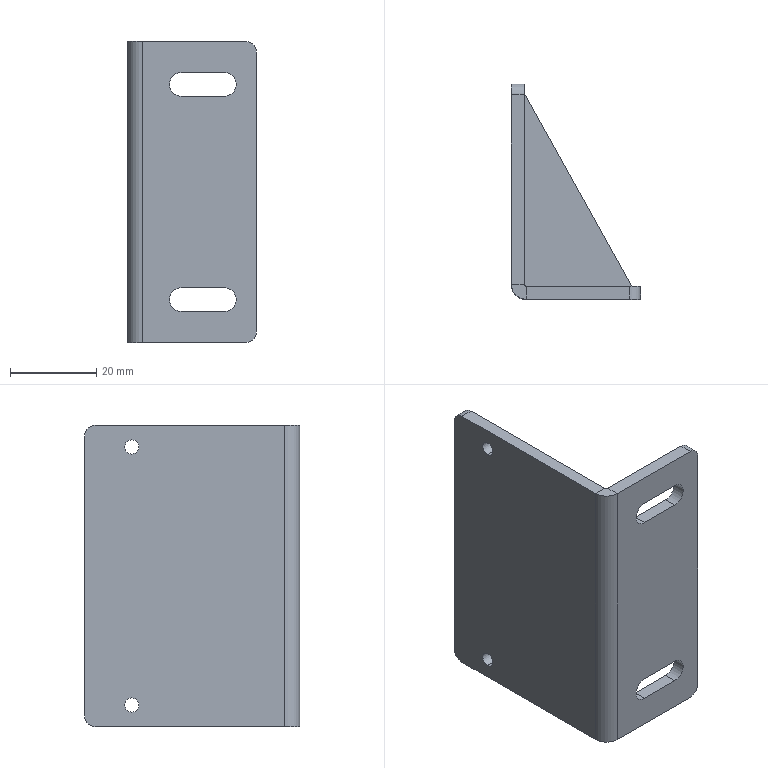Part | STEP file | KF-2212-070-007 | 2 solids | 35 faces | box 30 x 50 x 70 mm | volume 17137 mm3 | plane 21 | cylinder 14 | commonest cylinder face diameters 3.3 x4 5 x4 5.5 x4 1 x1 7 x1
STEP:
#1=CARTESIAN_POINT('',(3.,48.,36.5));
#2=VERTEX_POINT('',#1);
#3=CARTESIAN_POINT('',(28.,3.,36.5));
#4=VERTEX_POINT('',#3);
#5=CARTESIAN_POINT('',(3.,48.,36.5));
#6=DIRECTION('',(0.4856,-0.8742,0.));
#7=VECTOR('',#6,1000.);
#8=LINE('',#5,#7);
#9=EDGE_CURVE('',#2,#4,#8,.T.);
#10=ORIENTED_EDGE('',*,*,#9,.T.);
#11=CARTESIAN_POINT('',(28.,3.,33.5));
#12=VERTEX_POINT('',#11);
#13=CARTESIAN_POINT('',(28.,3.,33.5));
#14=DIRECTION('',(0.,0.,1.));
#15=VECTOR('',#14,1000.);
#16=LINE('',#13,#15);
#17=EDGE_CURVE('',#12,#4,#16,.T.);
#18=ORIENTED_EDGE('',*,*,#17,.F.);
#19=CARTESIAN_POINT('',(3.,48.,33.5));
#20=VERTEX_POINT('',#19);
#21=CARTESIAN_POINT('',(3.,48.,33.5));
#22=DIRECTION('',(0.4856,-0.8742,0.));
#23=VECTOR('',#22,1000.);
#24=LINE('',#21,#23);
#25=EDGE_CURVE('',#20,#12,#24,.T.);
#26=ORIENTED_EDGE('',*,*,#25,.F.);
#27=CARTESIAN_POINT('',(3.,48.,33.5));
#28=DIRECTION('',(0.,0.,1.));
#29=VECTOR('',#28,1000.);
#30=LINE('',#27,#29);
#31=EDGE_CURVE('',#20,#2,#30,.T.);
#32=ORIENTED_EDGE('',*,*,#31,.T.);
#33=EDGE_LOOP('',(#10,#18,#26,#32));
#34=FACE_OUTER_BOUND('',#33,.T.);
#35=CARTESIAN_POINT('',(3.,48.,33.5));
#36=DIRECTION('',(-0.8742,-0.4856,0.));
#37=DIRECTION('',(0.4856,-0.8742,0.));
#38=AXIS2_PLACEMENT_3D('',#35,#36,#37);
#39=PLANE('',#38);
#40=ADVANCED_FACE('',(#34),#39,.F.);
#41=CARTESIAN_POINT('',(3.,3.,36.5));
#42=VERTEX_POINT('',#41);
#43=CARTESIAN_POINT('',(3.,3.,36.5));
#44=DIRECTION('',(-1.,0.,0.));
#45=VECTOR('',#44,1000.);
#46=LINE('',#43,#45);
#47=EDGE_CURVE('',#4,#42,#46,.T.);
#48=ORIENTED_EDGE('',*,*,#47,.T.);
#49=CARTESIAN_POINT('',(3.,3.,33.5));
#50=VERTEX_POINT('',#49);
#51=CARTESIAN_POINT('',(3.,3.,33.5));
#52=DIRECTION('',(0.,0.,1.));
#53=VECTOR('',#52,1000.);
#54=LINE('',#51,#53);
#55=EDGE_CURVE('',#50,#42,#54,.T.);
#56=ORIENTED_EDGE('',*,*,#55,.F.);
#57=CARTESIAN_POINT('',(3.,3.,33.5));
#58=DIRECTION('',(-1.,0.,0.));
#59=VECTOR('',#58,1000.);
#60=LINE('',#57,#59);
#61=EDGE_CURVE('',#12,#50,#60,.T.);
#62=ORIENTED_EDGE('',*,*,#61,.F.);
#63=ORIENTED_EDGE('',*,*,#17,.T.);
#64=EDGE_LOOP('',(#48,#56,#62,#63));
#65=FACE_OUTER_BOUND('',#64,.T.);
#66=CARTESIAN_POINT('',(3.,3.,33.5));
#67=DIRECTION('',(0.,1.,0.));
#68=DIRECTION('',(0.,0.,1.));
#69=AXIS2_PLACEMENT_3D('',#66,#67,#68);
#70=PLANE('',#69);
#71=ADVANCED_FACE('',(#65),#70,.F.);
#72=CARTESIAN_POINT('',(3.,3.,36.5));
#73=DIRECTION('',(0.,1.,0.));
#74=VECTOR('',#73,1000.);
#75=LINE('',#72,#74);
#76=EDGE_CURVE('',#42,#2,#75,.T.);
#77=ORIENTED_EDGE('',*,*,#76,.T.);
#78=ORIENTED_EDGE('',*,*,#31,.F.);
#79=CARTESIAN_POINT('',(3.,3.,33.5));
#80=DIRECTION('',(0.,1.,0.));
#81=VECTOR('',#80,1000.);
#82=LINE('',#79,#81);
#83=EDGE_CURVE('',#50,#20,#82,.T.);
#84=ORIENTED_EDGE('',*,*,#83,.F.);
#85=ORIENTED_EDGE('',*,*,#55,.T.);
#86=EDGE_LOOP('',(#77,#78,#84,#85));
#87=FACE_OUTER_BOUND('',#86,.T.);
#88=CARTESIAN_POINT('',(3.,3.,33.5));
#89=DIRECTION('',(1.,0.,0.));
#90=DIRECTION('',(0.,0.,-1.));
#91=AXIS2_PLACEMENT_3D('',#88,#89,#90);
#92=PLANE('',#91);
#93=ADVANCED_FACE('',(#87),#92,.F.);
#94=ORIENTED_EDGE('',*,*,#25,.T.);
#95=ORIENTED_EDGE('',*,*,#61,.T.);
#96=ORIENTED_EDGE('',*,*,#83,.T.);
#97=EDGE_LOOP('',(#94,#95,#96));
#98=FACE_OUTER_BOUND('',#97,.T.);
#99=CARTESIAN_POINT('',(0.,0.,33.5));
#100=DIRECTION('',(0.,0.,1.));
#101=DIRECTION('',(1.,0.,0.));
#102=AXIS2_PLACEMENT_3D('',#99,#100,#101);
#103=PLANE('',#102);
#104=ADVANCED_FACE('',(#98),#103,.F.);
#105=ORIENTED_EDGE('',*,*,#9,.F.);
#106=ORIENTED_EDGE('',*,*,#76,.F.);
#107=ORIENTED_EDGE('',*,*,#47,.F.);
#108=EDGE_LOOP('',(#105,#106,#107));
#109=FACE_OUTER_BOUND('',#108,.T.);
#110=CARTESIAN_POINT('',(0.,0.,36.5));
#111=DIRECTION('',(0.,0.,1.));
#112=DIRECTION('',(1.,0.,0.));
#113=AXIS2_PLACEMENT_3D('',#110,#111,#112);
#114=PLANE('',#113);
#115=ADVANCED_FACE('',(#109),#114,.T.);
#116=CLOSED_SHELL('',(#40,#71,#93,#104,#115));
#117=MANIFOLD_SOLID_BREP('',#116);
#118=CARTESIAN_POINT('',(0.,39.,6.65));
#119=VERTEX_POINT('',#118);
#120=CARTESIAN_POINT('',(0.,39.,3.35));
#121=VERTEX_POINT('',#120);
#122=CARTESIAN_POINT('',(0.,39.,5.));
#123=DIRECTION('',(1.,0.,0.));
#124=DIRECTION('',(0.,0.,-1.));
#125=AXIS2_PLACEMENT_3D('',#122,#123,#124);
#126=CIRCLE('',#125,1.65);
#127=EDGE_CURVE('',#119,#121,#126,.T.);
#128=ORIENTED_EDGE('',*,*,#127,.F.);
#129=CARTESIAN_POINT('',(3.,39.,6.65));
#130=VERTEX_POINT('',#129);
#131=CARTESIAN_POINT('',(3.,39.,6.65));
#132=DIRECTION('',(1.,0.,0.));
#133=VECTOR('',#132,1000.);
#134=LINE('',#131,#133);
#135=EDGE_CURVE('',#119,#130,#134,.T.);
#136=ORIENTED_EDGE('',*,*,#135,.T.);
#137=CARTESIAN_POINT('',(3.,39.,3.35));
#138=VERTEX_POINT('',#137);
#139=CARTESIAN_POINT('',(3.,39.,5.));
#140=DIRECTION('',(1.,0.,0.));
#141=DIRECTION('',(0.,0.,-1.));
#142=AXIS2_PLACEMENT_3D('',#139,#140,#141);
#143=CIRCLE('',#142,1.65);
#144=EDGE_CURVE('',#130,#138,#143,.T.);
#145=ORIENTED_EDGE('',*,*,#144,.T.);
#146=CARTESIAN_POINT('',(3.,39.,3.35));
#147=DIRECTION('',(1.,0.,0.));
#148=VECTOR('',#147,1000.);
#149=LINE('',#146,#148);
#150=EDGE_CURVE('',#121,#138,#149,.T.);
#151=ORIENTED_EDGE('',*,*,#150,.F.);
#152=EDGE_LOOP('',(#128,#136,#145,#151));
#153=FACE_OUTER_BOUND('',#152,.T.);
#154=CARTESIAN_POINT('',(3.,39.,5.));
#155=DIRECTION('',(1.,0.,0.));
#156=DIRECTION('',(0.,0.,-1.));
#157=AXIS2_PLACEMENT_3D('',#154,#155,#156);
#158=CYLINDRICAL_SURFACE('',#157,1.65);
#159=ADVANCED_FACE('',(#153),#158,.F.);
#160=CARTESIAN_POINT('',(0.,39.,66.65));
#161=VERTEX_POINT('',#160);
#162=CARTESIAN_POINT('',(0.,39.,63.35));
#163=VERTEX_POINT('',#162);
#164=CARTESIAN_POINT('',(0.,39.,65.));
#165=DIRECTION('',(1.,0.,0.));
#166=DIRECTION('',(0.,0.,-1.));
#167=AXIS2_PLACEMENT_3D('',#164,#165,#166);
#168=CIRCLE('',#167,1.65);
#169=EDGE_CURVE('',#161,#163,#168,.T.);
#170=ORIENTED_EDGE('',*,*,#169,.F.);
#171=CARTESIAN_POINT('',(3.,39.,66.65));
#172=VERTEX_POINT('',#171);
#173=CARTESIAN_POINT('',(3.,39.,66.65));
#174=DIRECTION('',(1.,0.,0.));
#175=VECTOR('',#174,1000.);
#176=LINE('',#173,#175);
#177=EDGE_CURVE('',#161,#172,#176,.T.);
#178=ORIENTED_EDGE('',*,*,#177,.T.);
#179=CARTESIAN_POINT('',(3.,39.,63.35));
#180=VERTEX_POINT('',#179);
#181=CARTESIAN_POINT('',(3.,39.,65.));
#182=DIRECTION('',(1.,0.,0.));
#183=DIRECTION('',(0.,0.,-1.));
#184=AXIS2_PLACEMENT_3D('',#181,#182,#183);
#185=CIRCLE('',#184,1.65);
#186=EDGE_CURVE('',#172,#180,#185,.T.);
#187=ORIENTED_EDGE('',*,*,#186,.T.);
#188=CARTESIAN_POINT('',(3.,39.,63.35));
#189=DIRECTION('',(1.,0.,0.));
#190=VECTOR('',#189,1000.);
#191=LINE('',#188,#190);
#192=EDGE_CURVE('',#163,#180,#191,.T.);
#193=ORIENTED_EDGE('',*,*,#192,.F.);
#194=EDGE_LOOP('',(#170,#178,#187,#193));
#195=FACE_OUTER_BOUND('',#194,.T.);
#196=CARTESIAN_POINT('',(3.,39.,65.));
#197=DIRECTION('',(1.,0.,0.));
#198=DIRECTION('',(0.,0.,-1.));
#199=AXIS2_PLACEMENT_3D('',#196,#197,#198);
#200=CYLINDRICAL_SURFACE('',#199,1.65);
#201=ADVANCED_FACE('',(#195),#200,.F.);
#202=CARTESIAN_POINT('',(0.,3.5,70.));
#203=VERTEX_POINT('',#202);
#204=CARTESIAN_POINT('',(3.,3.5,70.));
#205=VERTEX_POINT('',#204);
#206=CARTESIAN_POINT('',(0.,3.5,70.));
#207=DIRECTION('',(1.,0.,0.));
#208=VECTOR('',#207,1000.);
#209=LINE('',#206,#208);
#210=EDGE_CURVE('',#203,#205,#209,.T.);
#211=ORIENTED_EDGE('',*,*,#210,.F.);
#212=CARTESIAN_POINT('',(3.5,0.,70.));
#213=VERTEX_POINT('',#212);
#214=CARTESIAN_POINT('',(3.5,3.5,70.));
#215=DIRECTION('',(0.,0.,1.));
#216=DIRECTION('',(-1.,0.,0.));
#217=AXIS2_PLACEMENT_3D('',#214,#215,#216);
#218=CIRCLE('',#217,3.5);
#219=EDGE_CURVE('',#203,#213,#218,.T.);
#220=ORIENTED_EDGE('',*,*,#219,.T.);
#221=CARTESIAN_POINT('',(3.5,3.,70.));
#222=VERTEX_POINT('',#221);
#223=CARTESIAN_POINT('',(3.5,3.,70.));
#224=DIRECTION('',(0.,-1.,0.));
#225=VECTOR('',#224,1000.);
#226=LINE('',#223,#225);
#227=EDGE_CURVE('',#222,#213,#226,.T.);
#228=ORIENTED_EDGE('',*,*,#227,.F.);
#229=CARTESIAN_POINT('',(3.5,3.5,70.));
#230=DIRECTION('',(0.,0.,1.));
#231=DIRECTION('',(1.,0.,0.));
#232=AXIS2_PLACEMENT_3D('',#229,#230,#231);
#233=CIRCLE('',#232,0.5);
#234=EDGE_CURVE('',#205,#222,#233,.T.);
#235=ORIENTED_EDGE('',*,*,#234,.F.);
#236=EDGE_LOOP('',(#211,#220,#228,#235));
#237=FACE_OUTER_BOUND('',#236,.T.);
#238=CARTESIAN_POINT('',(0.,3.5,70.));
#239=DIRECTION('',(0.,0.,1.));
#240=DIRECTION('',(1.,0.,0.));
#241=AXIS2_PLACEMENT_3D('',#238,#239,#240);
#242=PLANE('',#241);
#243=ADVANCED_FACE('',(#237),#242,.T.);
#244=CARTESIAN_POINT('',(3.,47.5,70.));
#245=VERTEX_POINT('',#244);
#246=CARTESIAN_POINT('',(3.,0.,70.));
#247=DIRECTION('',(0.,-1.,0.));
#248=VECTOR('',#247,1000.);
#249=LINE('',#246,#248);
#250=EDGE_CURVE('',#245,#205,#249,.T.);
#251=ORIENTED_EDGE('',*,*,#250,.F.);
#252=CARTESIAN_POINT('',(0.,47.5,70.));
#253=VERTEX_POINT('',#252);
#254=CARTESIAN_POINT('',(3.5,47.5,70.));
#255=DIRECTION('',(-1.,0.,0.));
#256=VECTOR('',#255,1000.);
#257=LINE('',#254,#256);
#258=EDGE_CURVE('',#245,#253,#257,.T.);
#259=ORIENTED_EDGE('',*,*,#258,.T.);
#260=CARTESIAN_POINT('',(0.,0.,70.));
#261=DIRECTION('',(0.,-1.,0.));
#262=VECTOR('',#261,1000.);
#263=LINE('',#260,#262);
#264=EDGE_CURVE('',#253,#203,#263,.T.);
#265=ORIENTED_EDGE('',*,*,#264,.T.);
#266=ORIENTED_EDGE('',*,*,#210,.T.);
#267=EDGE_LOOP('',(#251,#259,#265,#266));
#268=FACE_OUTER_BOUND('',#267,.T.);
#269=CARTESIAN_POINT('',(3.5,3.,70.));
#270=DIRECTION('',(0.,0.,1.));
#271=DIRECTION('',(1.,0.,0.));
#272=AXIS2_PLACEMENT_3D('',#269,#270,#271);
#273=PLANE('',#272);
#274=ADVANCED_FACE('',(#268),#273,.T.);
#275=CARTESIAN_POINT('',(3.5,0.,0.));
#276=VERTEX_POINT('',#275);
#277=CARTESIAN_POINT('',(3.5,3.,0.));
#278=VERTEX_POINT('',#277);
#279=CARTESIAN_POINT('',(3.5,0.,0.));
#280=DIRECTION('',(0.,1.,0.));
#281=VECTOR('',#280,1000.);
#282=LINE('',#279,#281);
#283=EDGE_CURVE('',#276,#278,#282,.T.);
#284=ORIENTED_EDGE('',*,*,#283,.F.);
#285=CARTESIAN_POINT('',(0.,3.5,0.));
#286=VERTEX_POINT('',#285);
#287=CARTESIAN_POINT('',(3.5,3.5,0.));
#288=DIRECTION('',(0.,0.,1.));
#289=DIRECTION('',(-1.,0.,0.));
#290=AXIS2_PLACEMENT_3D('',#287,#288,#289);
#291=CIRCLE('',#290,3.5);
#292=EDGE_CURVE('',#286,#276,#291,.T.);
#293=ORIENTED_EDGE('',*,*,#292,.F.);
#294=CARTESIAN_POINT('',(3.,3.5,0.));
#295=VERTEX_POINT('',#294);
#296=CARTESIAN_POINT('',(3.,3.5,0.));
#297=DIRECTION('',(-1.,0.,0.));
#298=VECTOR('',#297,1000.);
#299=LINE('',#296,#298);
#300=EDGE_CURVE('',#295,#286,#299,.T.);
#301=ORIENTED_EDGE('',*,*,#300,.F.);
#302=CARTESIAN_POINT('',(3.5,3.5,0.));
#303=DIRECTION('',(0.,0.,1.));
#304=DIRECTION('',(1.,0.,0.));
#305=AXIS2_PLACEMENT_3D('',#302,#303,#304);
#306=CIRCLE('',#305,0.5);
#307=EDGE_CURVE('',#295,#278,#306,.T.);
#308=ORIENTED_EDGE('',*,*,#307,.T.);
#309=EDGE_LOOP('',(#284,#293,#301,#308));
#310=FACE_OUTER_BOUND('',#309,.T.);
#311=CARTESIAN_POINT('',(3.5,0.,0.));
#312=DIRECTION('',(0.,0.,-1.));
#313=DIRECTION('',(-1.,0.,0.));
#314=AXIS2_PLACEMENT_3D('',#311,#312,#313);
#315=PLANE('',#314);
#316=ADVANCED_FACE('',(#310),#315,.T.);
#317=CARTESIAN_POINT('',(27.5,3.,0.));
#318=VERTEX_POINT('',#317);
#319=CARTESIAN_POINT('',(0.,3.,0.));
#320=DIRECTION('',(1.,0.,0.));
#321=VECTOR('',#320,1000.);
#322=LINE('',#319,#321);
#323=EDGE_CURVE('',#278,#318,#322,.T.);
#324=ORIENTED_EDGE('',*,*,#323,.T.);
#325=CARTESIAN_POINT('',(27.5,0.,0.));
#326=VERTEX_POINT('',#325);
#327=CARTESIAN_POINT('',(27.5,3.5,0.));
#328=DIRECTION('',(0.,-1.,0.));
#329=VECTOR('',#328,1000.);
#330=LINE('',#327,#329);
#331=EDGE_CURVE('',#318,#326,#330,.T.);
#332=ORIENTED_EDGE('',*,*,#331,.T.);
#333=CARTESIAN_POINT('',(0.,0.,0.));
#334=DIRECTION('',(1.,0.,0.));
#335=VECTOR('',#334,1000.);
#336=LINE('',#333,#335);
#337=EDGE_CURVE('',#276,#326,#336,.T.);
#338=ORIENTED_EDGE('',*,*,#337,.F.);
#339=ORIENTED_EDGE('',*,*,#283,.T.);
#340=EDGE_LOOP('',(#324,#332,#338,#339));
#341=FACE_OUTER_BOUND('',#340,.T.);
#342=CARTESIAN_POINT('',(3.,3.5,0.));
#343=DIRECTION('',(0.,0.,-1.));
#344=DIRECTION('',(-1.,0.,0.));
#345=AXIS2_PLACEMENT_3D('',#342,#343,#344);
#346=PLANE('',#345);
#347=ADVANCED_FACE('',(#341),#346,.T.);
#348=CARTESIAN_POINT('',(12.5,0.,7.25));
#349=VERTEX_POINT('',#348);
#350=CARTESIAN_POINT('',(22.5,0.,7.25));
#351=VERTEX_POINT('',#350);
#352=CARTESIAN_POINT('',(12.5,0.,7.25));
#353=DIRECTION('',(1.,0.,0.));
#354=VECTOR('',#353,1000.);
#355=LINE('',#352,#354);
#356=EDGE_CURVE('',#349,#351,#355,.T.);
#357=ORIENTED_EDGE('',*,*,#356,.F.);
#358=CARTESIAN_POINT('',(12.5,0.,12.75));
#359=VERTEX_POINT('',#358);
#360=CARTESIAN_POINT('',(12.5,0.,10.));
#361=DIRECTION('',(0.,-1.,0.));
#362=DIRECTION('',(0.,0.,-1.));
#363=AXIS2_PLACEMENT_3D('',#360,#361,#362);
#364=CIRCLE('',#363,2.75);
#365=EDGE_CURVE('',#359,#349,#364,.T.);
#366=ORIENTED_EDGE('',*,*,#365,.F.);
#367=CARTESIAN_POINT('',(22.5,0.,12.75));
#368=VERTEX_POINT('',#367);
#369=CARTESIAN_POINT('',(12.5,0.,12.75));
#370=DIRECTION('',(-1.,0.,0.));
#371=VECTOR('',#370,1000.);
#372=LINE('',#369,#371);
#373=EDGE_CURVE('',#368,#359,#372,.T.);
#374=ORIENTED_EDGE('',*,*,#373,.F.);
#375=CARTESIAN_POINT('',(22.5,0.,10.));
#376=DIRECTION('',(0.,-1.,0.));
#377=DIRECTION('',(0.,0.,-1.));
#378=AXIS2_PLACEMENT_3D('',#375,#376,#377);
#379=CIRCLE('',#378,2.75);
#380=EDGE_CURVE('',#351,#368,#379,.T.);
#381=ORIENTED_EDGE('',*,*,#380,.F.);
#382=EDGE_LOOP('',(#357,#366,#374,#381));
#383=FACE_BOUND('',#382,.T.);
#384=CARTESIAN_POINT('',(12.5,0.,57.25));
#385=VERTEX_POINT('',#384);
#386=CARTESIAN_POINT('',(22.5,0.,57.25));
#387=VERTEX_POINT('',#386);
#388=CARTESIAN_POINT('',(12.5,0.,57.25));
#389=DIRECTION('',(1.,0.,0.));
#390=VECTOR('',#389,1000.);
#391=LINE('',#388,#390);
#392=EDGE_CURVE('',#385,#387,#391,.T.);
#393=ORIENTED_EDGE('',*,*,#392,.F.);
#394=CARTESIAN_POINT('',(12.5,0.,62.75));
#395=VERTEX_POINT('',#394);
#396=CARTESIAN_POINT('',(12.5,0.,60.));
#397=DIRECTION('',(0.,-1.,0.));
#398=DIRECTION('',(0.,0.,-1.));
#399=AXIS2_PLACEMENT_3D('',#396,#397,#398);
#400=CIRCLE('',#399,2.75);
#401=EDGE_CURVE('',#395,#385,#400,.T.);
#402=ORIENTED_EDGE('',*,*,#401,.F.);
#403=CARTESIAN_POINT('',(22.5,0.,62.75));
#404=VERTEX_POINT('',#403);
#405=CARTESIAN_POINT('',(12.5,0.,62.75));
#406=DIRECTION('',(-1.,0.,0.));
#407=VECTOR('',#406,1000.);
#408=LINE('',#405,#407);
#409=EDGE_CURVE('',#404,#395,#408,.T.);
#410=ORIENTED_EDGE('',*,*,#409,.F.);
#411=CARTESIAN_POINT('',(22.5,0.,60.));
#412=DIRECTION('',(0.,-1.,0.));
#413=DIRECTION('',(0.,0.,-1.));
#414=AXIS2_PLACEMENT_3D('',#411,#412,#413);
#415=CIRCLE('',#414,2.75);
#416=EDGE_CURVE('',#387,#404,#415,.T.);
#417=ORIENTED_EDGE('',*,*,#416,.F.);
#418=EDGE_LOOP('',(#393,#402,#410,#417));
#419=FACE_BOUND('',#418,.T.);
#420=ORIENTED_EDGE('',*,*,#337,.T.);
#421=CARTESIAN_POINT('',(30.,0.,2.5));
#422=VERTEX_POINT('',#421);
#423=CARTESIAN_POINT('',(27.5,0.,2.5));
#424=DIRECTION('',(0.,-1.,0.));
#425=DIRECTION('',(0.,0.,1.));
#426=AXIS2_PLACEMENT_3D('',#423,#424,#425);
#427=CIRCLE('',#426,2.5);
#428=EDGE_CURVE('',#326,#422,#427,.T.);
#429=ORIENTED_EDGE('',*,*,#428,.T.);
#430=CARTESIAN_POINT('',(30.,0.,67.5));
#431=VERTEX_POINT('',#430);
#432=CARTESIAN_POINT('',(30.,0.,70.));
#433=DIRECTION('',(0.,0.,-1.));
#434=VECTOR('',#433,1000.);
#435=LINE('',#432,#434);
#436=EDGE_CURVE('',#431,#422,#435,.T.);
#437=ORIENTED_EDGE('',*,*,#436,.F.);
#438=CARTESIAN_POINT('',(27.5,0.,70.));
#439=VERTEX_POINT('',#438);
#440=CARTESIAN_POINT('',(27.5,0.,67.5));
#441=DIRECTION('',(0.,-1.,0.));
#442=DIRECTION('',(0.,0.,1.));
#443=AXIS2_PLACEMENT_3D('',#440,#441,#442);
#444=CIRCLE('',#443,2.5);
#445=EDGE_CURVE('',#431,#439,#444,.T.);
#446=ORIENTED_EDGE('',*,*,#445,.T.);
#447=CARTESIAN_POINT('',(0.,0.,70.));
#448=DIRECTION('',(1.,0.,0.));
#449=VECTOR('',#448,1000.);
#450=LINE('',#447,#449);
#451=EDGE_CURVE('',#213,#439,#450,.T.);
#452=ORIENTED_EDGE('',*,*,#451,.F.);
#453=CARTESIAN_POINT('',(3.5,0.,70.));
#454=DIRECTION('',(0.,0.,-1.));
#455=VECTOR('',#454,1000.);
#456=LINE('',#453,#455);
#457=EDGE_CURVE('',#213,#276,#456,.T.);
#458=ORIENTED_EDGE('',*,*,#457,.T.);
#459=EDGE_LOOP('',(#420,#429,#437,#446,#452,#458));
#460=FACE_OUTER_BOUND('',#459,.T.);
#461=CARTESIAN_POINT('',(0.,0.,70.));
#462=DIRECTION('',(0.,1.,0.));
#463=DIRECTION('',(0.,0.,1.));
#464=AXIS2_PLACEMENT_3D('',#461,#462,#463);
#465=PLANE('',#464);
#466=ADVANCED_FACE('',(#383,#419,#460),#465,.F.);
#467=ORIENTED_EDGE('',*,*,#436,.T.);
#468=CARTESIAN_POINT('',(30.,3.,2.5));
#469=VERTEX_POINT('',#468);
#470=CARTESIAN_POINT('',(30.,3.,2.5));
#471=DIRECTION('',(0.,1.,0.));
#472=VECTOR('',#471,1000.);
#473=LINE('',#470,#472);
#474=EDGE_CURVE('',#422,#469,#473,.T.);
#475=ORIENTED_EDGE('',*,*,#474,.T.);
#476=CARTESIAN_POINT('',(30.,3.,67.5));
#477=VERTEX_POINT('',#476);
#478=CARTESIAN_POINT('',(30.,3.,70.));
#479=DIRECTION('',(0.,0.,-1.));
#480=VECTOR('',#479,1000.);
#481=LINE('',#478,#480);
#482=EDGE_CURVE('',#477,#469,#481,.T.);
#483=ORIENTED_EDGE('',*,*,#482,.F.);
#484=CARTESIAN_POINT('',(30.,3.,67.5));
#485=DIRECTION('',(0.,-1.,0.));
#486=VECTOR('',#485,1000.);
#487=LINE('',#484,#486);
#488=EDGE_CURVE('',#477,#431,#487,.T.);
#489=ORIENTED_EDGE('',*,*,#488,.T.);
#490=EDGE_LOOP('',(#467,#475,#483,#489));
#491=FACE_OUTER_BOUND('',#490,.T.);
#492=CARTESIAN_POINT('',(30.,3.,70.));
#493=DIRECTION('',(1.,0.,0.));
#494=DIRECTION('',(0.,0.,-1.));
#495=AXIS2_PLACEMENT_3D('',#492,#493,#494);
#496=PLANE('',#495);
#497=ADVANCED_FACE('',(#491),#496,.T.);
#498=CARTESIAN_POINT('',(12.5,3.,7.25));
#499=VERTEX_POINT('',#498);
#500=CARTESIAN_POINT('',(12.5,3.,12.75));
#501=VERTEX_POINT('',#500);
#502=CARTESIAN_POINT('',(12.5,3.,10.));
#503=DIRECTION('',(0.,1.,0.));
#504=DIRECTION('',(0.,0.,1.));
#505=AXIS2_PLACEMENT_3D('',#502,#503,#504);
#506=CIRCLE('',#505,2.75);
#507=EDGE_CURVE('',#499,#501,#506,.T.);
#508=ORIENTED_EDGE('',*,*,#507,.F.);
#509=CARTESIAN_POINT('',(22.5,3.,7.25));
#510=VERTEX_POINT('',#509);
#511=CARTESIAN_POINT('',(0.,3.,7.25));
#512=DIRECTION('',(-1.,0.,0.));
#513=VECTOR('',#512,1000.);
#514=LINE('',#511,#513);
#515=EDGE_CURVE('',#510,#499,#514,.T.);
#516=ORIENTED_EDGE('',*,*,#515,.F.);
#517=CARTESIAN_POINT('',(22.5,3.,12.75));
#518=VERTEX_POINT('',#517);
#519=CARTESIAN_POINT('',(22.5,3.,10.));
#520=DIRECTION('',(0.,1.,0.));
#521=DIRECTION('',(0.,0.,1.));
#522=AXIS2_PLACEMENT_3D('',#519,#520,#521);
#523=CIRCLE('',#522,2.75);
#524=EDGE_CURVE('',#518,#510,#523,.T.);
#525=ORIENTED_EDGE('',*,*,#524,.F.);
#526=CARTESIAN_POINT('',(0.,3.,12.75));
#527=DIRECTION('',(1.,0.,0.));
#528=VECTOR('',#527,1000.);
#529=LINE('',#526,#528);
#530=EDGE_CURVE('',#501,#518,#529,.T.);
#531=ORIENTED_EDGE('',*,*,#530,.F.);
#532=EDGE_LOOP('',(#508,#516,#525,#531));
#533=FACE_BOUND('',#532,.T.);
#534=CARTESIAN_POINT('',(12.5,3.,57.25));
#535=VERTEX_POINT('',#534);
#536=CARTESIAN_POINT('',(12.5,3.,62.75));
#537=VERTEX_POINT('',#536);
#538=CARTESIAN_POINT('',(12.5,3.,60.));
#539=DIRECTION('',(0.,1.,0.));
#540=DIRECTION('',(0.,0.,1.));
#541=AXIS2_PLACEMENT_3D('',#538,#539,#540);
#542=CIRCLE('',#541,2.75);
#543=EDGE_CURVE('',#535,#537,#542,.T.);
#544=ORIENTED_EDGE('',*,*,#543,.F.);
#545=CARTESIAN_POINT('',(22.5,3.,57.25));
#546=VERTEX_POINT('',#545);
#547=CARTESIAN_POINT('',(0.,3.,57.25));
#548=DIRECTION('',(-1.,0.,0.));
#549=VECTOR('',#548,1000.);
#550=LINE('',#547,#549);
#551=EDGE_CURVE('',#546,#535,#550,.T.);
#552=ORIENTED_EDGE('',*,*,#551,.F.);
#553=CARTESIAN_POINT('',(22.5,3.,62.75));
#554=VERTEX_POINT('',#553);
#555=CARTESIAN_POINT('',(22.5,3.,60.));
#556=DIRECTION('',(0.,1.,0.));
#557=DIRECTION('',(0.,0.,1.));
#558=AXIS2_PLACEMENT_3D('',#555,#556,#557);
#559=CIRCLE('',#558,2.75);
#560=EDGE_CURVE('',#554,#546,#559,.T.);
#561=ORIENTED_EDGE('',*,*,#560,.F.);
#562=CARTESIAN_POINT('',(0.,3.,62.75));
#563=DIRECTION('',(1.,0.,0.));
#564=VECTOR('',#563,1000.);
#565=LINE('',#562,#564);
#566=EDGE_CURVE('',#537,#554,#565,.T.);
#567=ORIENTED_EDGE('',*,*,#566,.F.);
#568=EDGE_LOOP('',(#544,#552,#561,#567));
#569=FACE_BOUND('',#568,.T.);
#570=ORIENTED_EDGE('',*,*,#482,.T.);
#571=CARTESIAN_POINT('',(27.5,3.,2.5));
#572=DIRECTION('',(0.,1.,0.));
#573=DIRECTION('',(0.,0.,1.));
#574=AXIS2_PLACEMENT_3D('',#571,#572,#573);
#575=CIRCLE('',#574,2.5);
#576=EDGE_CURVE('',#469,#318,#575,.T.);
#577=ORIENTED_EDGE('',*,*,#576,.T.);
#578=ORIENTED_EDGE('',*,*,#323,.F.);
#579=CARTESIAN_POINT('',(3.5,3.,70.));
#580=DIRECTION('',(0.,0.,-1.));
#581=VECTOR('',#580,1000.);
#582=LINE('',#579,#581);
#583=EDGE_CURVE('',#222,#278,#582,.T.);
#584=ORIENTED_EDGE('',*,*,#583,.F.);
#585=CARTESIAN_POINT('',(27.5,3.,70.));
#586=VERTEX_POINT('',#585);
#587=CARTESIAN_POINT('',(0.,3.,70.));
#588=DIRECTION('',(1.,0.,0.));
#589=VECTOR('',#588,1000.);
#590=LINE('',#587,#589);
#591=EDGE_CURVE('',#222,#586,#590,.T.);
#592=ORIENTED_EDGE('',*,*,#591,.T.);
#593=CARTESIAN_POINT('',(27.5,3.,67.5));
#594=DIRECTION('',(0.,1.,0.));
#595=DIRECTION('',(0.,0.,1.));
#596=AXIS2_PLACEMENT_3D('',#593,#594,#595);
#597=CIRCLE('',#596,2.5);
#598=EDGE_CURVE('',#586,#477,#597,.T.);
#599=ORIENTED_EDGE('',*,*,#598,.T.);
#600=EDGE_LOOP('',(#570,#577,#578,#584,#592,#599));
#601=FACE_OUTER_BOUND('',#600,.T.);
#602=CARTESIAN_POINT('',(0.,3.,70.));
#603=DIRECTION('',(0.,1.,0.));
#604=DIRECTION('',(0.,0.,1.));
#605=AXIS2_PLACEMENT_3D('',#602,#603,#604);
#606=PLANE('',#605);
#607=ADVANCED_FACE('',(#533,#569,#601),#606,.T.);
#608=ORIENTED_EDGE('',*,*,#307,.F.);
#609=CARTESIAN_POINT('',(3.,3.5,70.));
#610=DIRECTION('',(0.,0.,-1.));
#611=VECTOR('',#610,1000.);
#612=LINE('',#609,#611);
#613=EDGE_CURVE('',#205,#295,#612,.T.);
#614=ORIENTED_EDGE('',*,*,#613,.F.);
#615=ORIENTED_EDGE('',*,*,#234,.T.);
#616=ORIENTED_EDGE('',*,*,#583,.T.);
#617=EDGE_LOOP('',(#608,#614,#615,#616));
#618=FACE_OUTER_BOUND('',#617,.T.);
#619=CARTESIAN_POINT('',(3.5,3.5,70.));
#620=DIRECTION('',(0.,0.,-1.));
#621=DIRECTION('',(-1.,0.,0.));
#622=AXIS2_PLACEMENT_3D('',#619,#620,#621);
#623=CYLINDRICAL_SURFACE('',#622,0.5);
#624=ADVANCED_FACE('',(#618),#623,.F.);
#625=CARTESIAN_POINT('',(3.,39.,5.));
#626=DIRECTION('',(1.,0.,0.));
#627=DIRECTION('',(0.,0.,-1.));
#628=AXIS2_PLACEMENT_3D('',#625,#626,#627);
#629=CIRCLE('',#628,1.65);
#630=EDGE_CURVE('',#138,#130,#629,.T.);
#631=ORIENTED_EDGE('',*,*,#630,.F.);
#632=ORIENTED_EDGE('',*,*,#144,.F.);
#633=EDGE_LOOP('',(#631,#632));
#634=FACE_BOUND('',#633,.T.);
#635=CARTESIAN_POINT('',(3.,39.,65.));
#636=DIRECTION('',(1.,0.,0.));
#637=DIRECTION('',(0.,0.,-1.));
#638=AXIS2_PLACEMENT_3D('',#635,#636,#637);
#639=CIRCLE('',#638,1.65);
#640=EDGE_CURVE('',#180,#172,#639,.T.);
#641=ORIENTED_EDGE('',*,*,#640,.F.);
#642=ORIENTED_EDGE('',*,*,#186,.F.);
#643=EDGE_LOOP('',(#641,#642));
#644=FACE_BOUND('',#643,.T.);
#645=CARTESIAN_POINT('',(3.,50.,67.5));
#646=VERTEX_POINT('',#645);
#647=CARTESIAN_POINT('',(3.,50.,2.5));
#648=VERTEX_POINT('',#647);
#649=CARTESIAN_POINT('',(3.,50.,70.));
#650=DIRECTION('',(0.,0.,-1.));
#651=VECTOR('',#650,1000.);
#652=LINE('',#649,#651);
#653=EDGE_CURVE('',#646,#648,#652,.T.);
#654=ORIENTED_EDGE('',*,*,#653,.F.);
#655=CARTESIAN_POINT('',(3.,47.5,67.5));
#656=DIRECTION('',(1.,0.,0.));
#657=DIRECTION('',(0.,0.,-1.));
#658=AXIS2_PLACEMENT_3D('',#655,#656,#657);
#659=CIRCLE('',#658,2.5);
#660=EDGE_CURVE('',#646,#245,#659,.T.);
#661=ORIENTED_EDGE('',*,*,#660,.T.);
#662=ORIENTED_EDGE('',*,*,#250,.T.);
#663=ORIENTED_EDGE('',*,*,#613,.T.);
#664=CARTESIAN_POINT('',(3.,47.5,0.));
#665=VERTEX_POINT('',#664);
#666=CARTESIAN_POINT('',(3.,0.,0.));
#667=DIRECTION('',(0.,-1.,0.));
#668=VECTOR('',#667,1000.);
#669=LINE('',#666,#668);
#670=EDGE_CURVE('',#665,#295,#669,.T.);
#671=ORIENTED_EDGE('',*,*,#670,.F.);
#672=CARTESIAN_POINT('',(3.,47.5,2.5));
#673=DIRECTION('',(1.,0.,0.));
#674=DIRECTION('',(0.,0.,-1.));
#675=AXIS2_PLACEMENT_3D('',#672,#673,#674);
#676=CIRCLE('',#675,2.5);
#677=EDGE_CURVE('',#665,#648,#676,.T.);
#678=ORIENTED_EDGE('',*,*,#677,.T.);
#679=EDGE_LOOP('',(#654,#661,#662,#663,#671,#678));
#680=FACE_OUTER_BOUND('',#679,.T.);
#681=CARTESIAN_POINT('',(3.,0.,70.));
#682=DIRECTION('',(1.,0.,0.));
#683=DIRECTION('',(0.,0.,-1.));
#684=AXIS2_PLACEMENT_3D('',#681,#682,#683);
#685=PLANE('',#684);
#686=ADVANCED_FACE('',(#634,#644,#680),#685,.T.);
#687=CARTESIAN_POINT('',(0.,50.,67.5));
#688=VERTEX_POINT('',#687);
#689=CARTESIAN_POINT('',(0.,50.,2.5));
#690=VERTEX_POINT('',#689);
#691=CARTESIAN_POINT('',(0.,50.,70.));
#692=DIRECTION('',(0.,0.,-1.));
#693=VECTOR('',#692,1000.);
#694=LINE('',#691,#693);
#695=EDGE_CURVE('',#688,#690,#694,.T.);
#696=ORIENTED_EDGE('',*,*,#695,.F.);
#697=CARTESIAN_POINT('',(0.,50.,67.5));
#698=DIRECTION('',(1.,0.,0.));
#699=VECTOR('',#698,1000.);
#700=LINE('',#697,#699);
#701=EDGE_CURVE('',#688,#646,#700,.T.);
#702=ORIENTED_EDGE('',*,*,#701,.T.);
#703=ORIENTED_EDGE('',*,*,#653,.T.);
#704=CARTESIAN_POINT('',(0.,50.,2.5));
#705=DIRECTION('',(-1.,0.,0.));
#706=VECTOR('',#705,1000.);
#707=LINE('',#704,#706);
#708=EDGE_CURVE('',#648,#690,#707,.T.);
#709=ORIENTED_EDGE('',*,*,#708,.T.);
#710=EDGE_LOOP('',(#696,#702,#703,#709));
#711=FACE_OUTER_BOUND('',#710,.T.);
#712=CARTESIAN_POINT('',(0.,50.,70.));
#713=DIRECTION('',(0.,1.,0.));
#714=DIRECTION('',(0.,0.,1.));
#715=AXIS2_PLACEMENT_3D('',#712,#713,#714);
#716=PLANE('',#715);
#717=ADVANCED_FACE('',(#711),#716,.T.);
#718=CARTESIAN_POINT('',(0.,39.,5.));
#719=DIRECTION('',(1.,0.,0.));
#720=DIRECTION('',(0.,0.,-1.));
#721=AXIS2_PLACEMENT_3D('',#718,#719,#720);
#722=CIRCLE('',#721,1.65);
#723=EDGE_CURVE('',#121,#119,#722,.T.);
#724=ORIENTED_EDGE('',*,*,#723,.T.);
#725=ORIENTED_EDGE('',*,*,#127,.T.);
#726=EDGE_LOOP('',(#724,#725));
#727=FACE_BOUND('',#726,.T.);
#728=CARTESIAN_POINT('',(0.,39.,65.));
#729=DIRECTION('',(1.,0.,0.));
#730=DIRECTION('',(0.,0.,-1.));
#731=AXIS2_PLACEMENT_3D('',#728,#729,#730);
#732=CIRCLE('',#731,1.65);
#733=EDGE_CURVE('',#163,#161,#732,.T.);
#734=ORIENTED_EDGE('',*,*,#733,.T.);
#735=ORIENTED_EDGE('',*,*,#169,.T.);
#736=EDGE_LOOP('',(#734,#735));
#737=FACE_BOUND('',#736,.T.);
#738=ORIENTED_EDGE('',*,*,#264,.F.);
#739=CARTESIAN_POINT('',(0.,47.5,67.5));
#740=DIRECTION('',(-1.,0.,0.));
#741=DIRECTION('',(0.,0.,-1.));
#742=AXIS2_PLACEMENT_3D('',#739,#740,#741);
#743=CIRCLE('',#742,2.5);
#744=EDGE_CURVE('',#253,#688,#743,.T.);
#745=ORIENTED_EDGE('',*,*,#744,.T.);
#746=ORIENTED_EDGE('',*,*,#695,.T.);
#747=CARTESIAN_POINT('',(0.,47.5,0.));
#748=VERTEX_POINT('',#747);
#749=CARTESIAN_POINT('',(0.,47.5,2.5));
#750=DIRECTION('',(-1.,0.,0.));
#751=DIRECTION('',(0.,0.,-1.));
#752=AXIS2_PLACEMENT_3D('',#749,#750,#751);
#753=CIRCLE('',#752,2.5);
#754=EDGE_CURVE('',#690,#748,#753,.T.);
#755=ORIENTED_EDGE('',*,*,#754,.T.);
#756=CARTESIAN_POINT('',(0.,0.,0.));
#757=DIRECTION('',(0.,-1.,0.));
#758=VECTOR('',#757,1000.);
#759=LINE('',#756,#758);
#760=EDGE_CURVE('',#748,#286,#759,.T.);
#761=ORIENTED_EDGE('',*,*,#760,.T.);
#762=CARTESIAN_POINT('',(0.,3.5,70.));
#763=DIRECTION('',(0.,0.,-1.));
#764=VECTOR('',#763,1000.);
#765=LINE('',#762,#764);
#766=EDGE_CURVE('',#203,#286,#765,.T.);
#767=ORIENTED_EDGE('',*,*,#766,.F.);
#768=EDGE_LOOP('',(#738,#745,#746,#755,#761,#767));
#769=FACE_OUTER_BOUND('',#768,.T.);
#770=CARTESIAN_POINT('',(0.,0.,70.));
#771=DIRECTION('',(1.,0.,0.));
#772=DIRECTION('',(0.,0.,-1.));
#773=AXIS2_PLACEMENT_3D('',#770,#771,#772);
#774=PLANE('',#773);
#775=ADVANCED_FACE('',(#727,#737,#769),#774,.F.);
#776=ORIENTED_EDGE('',*,*,#292,.T.);
#777=ORIENTED_EDGE('',*,*,#457,.F.);
#778=ORIENTED_EDGE('',*,*,#219,.F.);
#779=ORIENTED_EDGE('',*,*,#766,.T.);
#780=EDGE_LOOP('',(#776,#777,#778,#779));
#781=FACE_OUTER_BOUND('',#780,.T.);
#782=CARTESIAN_POINT('',(3.5,3.5,70.));
#783=DIRECTION('',(0.,0.,-1.));
#784=DIRECTION('',(-1.,0.,0.));
#785=AXIS2_PLACEMENT_3D('',#782,#783,#784);
#786=CYLINDRICAL_SURFACE('',#785,3.5);
#787=ADVANCED_FACE('',(#781),#786,.T.);
#788=ORIENTED_EDGE('',*,*,#451,.T.);
#789=CARTESIAN_POINT('',(27.5,3.5,70.));
#790=DIRECTION('',(0.,1.,0.));
#791=VECTOR('',#790,1000.);
#792=LINE('',#789,#791);
#793=EDGE_CURVE('',#439,#586,#792,.T.);
#794=ORIENTED_EDGE('',*,*,#793,.T.);
#795=ORIENTED_EDGE('',*,*,#591,.F.);
#796=ORIENTED_EDGE('',*,*,#227,.T.);
#797=EDGE_LOOP('',(#788,#794,#795,#796));
#798=FACE_OUTER_BOUND('',#797,.T.);
#799=CARTESIAN_POINT('',(3.5,3.5,70.));
#800=DIRECTION('',(0.,0.,1.));
#801=DIRECTION('',(1.,0.,0.));
#802=AXIS2_PLACEMENT_3D('',#799,#800,#801);
#803=PLANE('',#802);
#804=ADVANCED_FACE('',(#798),#803,.T.);
#805=ORIENTED_EDGE('',*,*,#760,.F.);
#806=CARTESIAN_POINT('',(3.,47.5,0.));
#807=DIRECTION('',(1.,0.,0.));
#808=VECTOR('',#807,1000.);
#809=LINE('',#806,#808);
#810=EDGE_CURVE('',#748,#665,#809,.T.);
#811=ORIENTED_EDGE('',*,*,#810,.T.);
#812=ORIENTED_EDGE('',*,*,#670,.T.);
#813=ORIENTED_EDGE('',*,*,#300,.T.);
#814=EDGE_LOOP('',(#805,#811,#812,#813));
#815=FACE_OUTER_BOUND('',#814,.T.);
#816=CARTESIAN_POINT('',(3.5,3.5,0.));
#817=DIRECTION('',(0.,0.,1.));
#818=DIRECTION('',(1.,0.,0.));
#819=AXIS2_PLACEMENT_3D('',#816,#817,#818);
#820=PLANE('',#819);
#821=ADVANCED_FACE('',(#815),#820,.F.);
#822=ORIENTED_EDGE('',*,*,#576,.F.);
#823=ORIENTED_EDGE('',*,*,#474,.F.);
#824=ORIENTED_EDGE('',*,*,#428,.F.);
#825=ORIENTED_EDGE('',*,*,#331,.F.);
#826=EDGE_LOOP('',(#822,#823,#824,#825));
#827=FACE_OUTER_BOUND('',#826,.T.);
#828=CARTESIAN_POINT('',(27.5,3.5,2.5));
#829=DIRECTION('',(0.,-1.,0.));
#830=DIRECTION('',(0.,0.,-1.));
#831=AXIS2_PLACEMENT_3D('',#828,#829,#830);
#832=CYLINDRICAL_SURFACE('',#831,2.5);
#833=ADVANCED_FACE('',(#827),#832,.T.);
#834=ORIENTED_EDGE('',*,*,#598,.F.);
#835=ORIENTED_EDGE('',*,*,#793,.F.);
#836=ORIENTED_EDGE('',*,*,#445,.F.);
#837=ORIENTED_EDGE('',*,*,#488,.F.);
#838=EDGE_LOOP('',(#834,#835,#836,#837));
#839=FACE_OUTER_BOUND('',#838,.T.);
#840=CARTESIAN_POINT('',(27.5,3.,67.5));
#841=DIRECTION('',(0.,-1.,0.));
#842=DIRECTION('',(0.,0.,-1.));
#843=AXIS2_PLACEMENT_3D('',#840,#841,#842);
#844=CYLINDRICAL_SURFACE('',#843,2.5);
#845=ADVANCED_FACE('',(#839),#844,.T.);
#846=ORIENTED_EDGE('',*,*,#744,.F.);
#847=ORIENTED_EDGE('',*,*,#258,.F.);
#848=ORIENTED_EDGE('',*,*,#660,.F.);
#849=ORIENTED_EDGE('',*,*,#701,.F.);
#850=EDGE_LOOP('',(#846,#847,#848,#849));
#851=FACE_OUTER_BOUND('',#850,.T.);
#852=CARTESIAN_POINT('',(0.,47.5,67.5));
#853=DIRECTION('',(1.,0.,0.));
#854=DIRECTION('',(0.,0.,-1.));
#855=AXIS2_PLACEMENT_3D('',#852,#853,#854);
#856=CYLINDRICAL_SURFACE('',#855,2.5);
#857=ADVANCED_FACE('',(#851),#856,.T.);
#858=ORIENTED_EDGE('',*,*,#754,.F.);
#859=ORIENTED_EDGE('',*,*,#708,.F.);
#860=ORIENTED_EDGE('',*,*,#677,.F.);
#861=ORIENTED_EDGE('',*,*,#810,.F.);
#862=EDGE_LOOP('',(#858,#859,#860,#861));
#863=FACE_OUTER_BOUND('',#862,.T.);
#864=CARTESIAN_POINT('',(3.5,47.5,2.5));
#865=DIRECTION('',(-1.,0.,0.));
#866=DIRECTION('',(0.,0.,1.));
#867=AXIS2_PLACEMENT_3D('',#864,#865,#866);
#868=CYLINDRICAL_SURFACE('',#867,2.5);
#869=ADVANCED_FACE('',(#863),#868,.T.);
#870=ORIENTED_EDGE('',*,*,#543,.T.);
#871=CARTESIAN_POINT('',(12.5,10.,62.75));
#872=DIRECTION('',(0.,-1.,0.));
#873=VECTOR('',#872,1000.);
#874=LINE('',#871,#873);
#875=EDGE_CURVE('',#537,#395,#874,.T.);
#876=ORIENTED_EDGE('',*,*,#875,.T.);
#877=ORIENTED_EDGE('',*,*,#401,.T.);
#878=CARTESIAN_POINT('',(12.5,10.,57.25));
#879=DIRECTION('',(0.,-1.,0.));
#880=VECTOR('',#879,1000.);
#881=LINE('',#878,#880);
#882=EDGE_CURVE('',#535,#385,#881,.T.);
#883=ORIENTED_EDGE('',*,*,#882,.F.);
#884=EDGE_LOOP('',(#870,#876,#877,#883));
#885=FACE_OUTER_BOUND('',#884,.T.);
#886=CARTESIAN_POINT('',(12.5,10.,60.));
#887=DIRECTION('',(0.,-1.,0.));
#888=DIRECTION('',(0.,0.,-1.));
#889=AXIS2_PLACEMENT_3D('',#886,#887,#888);
#890=CYLINDRICAL_SURFACE('',#889,2.75);
#891=ADVANCED_FACE('',(#885),#890,.F.);
#892=ORIENTED_EDGE('',*,*,#566,.T.);
#893=CARTESIAN_POINT('',(22.5,10.,62.75));
#894=DIRECTION('',(0.,-1.,0.));
#895=VECTOR('',#894,1000.);
#896=LINE('',#893,#895);
#897=EDGE_CURVE('',#554,#404,#896,.T.);
#898=ORIENTED_EDGE('',*,*,#897,.T.);
#899=ORIENTED_EDGE('',*,*,#409,.T.);
#900=ORIENTED_EDGE('',*,*,#875,.F.);
#901=EDGE_LOOP('',(#892,#898,#899,#900));
#902=FACE_OUTER_BOUND('',#901,.T.);
#903=CARTESIAN_POINT('',(12.5,10.,62.75));
#904=DIRECTION('',(0.,0.,1.));
#905=DIRECTION('',(1.,0.,0.));
#906=AXIS2_PLACEMENT_3D('',#903,#904,#905);
#907=PLANE('',#906);
#908=ADVANCED_FACE('',(#902),#907,.F.);
#909=ORIENTED_EDGE('',*,*,#560,.T.);
#910=CARTESIAN_POINT('',(22.5,10.,57.25));
#911=DIRECTION('',(0.,-1.,0.));
#912=VECTOR('',#911,1000.);
#913=LINE('',#910,#912);
#914=EDGE_CURVE('',#546,#387,#913,.T.);
#915=ORIENTED_EDGE('',*,*,#914,.T.);
#916=ORIENTED_EDGE('',*,*,#416,.T.);
#917=ORIENTED_EDGE('',*,*,#897,.F.);
#918=EDGE_LOOP('',(#909,#915,#916,#917));
#919=FACE_OUTER_BOUND('',#918,.T.);
#920=CARTESIAN_POINT('',(22.5,10.,60.));
#921=DIRECTION('',(0.,-1.,0.));
#922=DIRECTION('',(0.,0.,-1.));
#923=AXIS2_PLACEMENT_3D('',#920,#921,#922);
#924=CYLINDRICAL_SURFACE('',#923,2.75);
#925=ADVANCED_FACE('',(#919),#924,.F.);
#926=ORIENTED_EDGE('',*,*,#551,.T.);
#927=ORIENTED_EDGE('',*,*,#882,.T.);
#928=ORIENTED_EDGE('',*,*,#392,.T.);
#929=ORIENTED_EDGE('',*,*,#914,.F.);
#930=EDGE_LOOP('',(#926,#927,#928,#929));
#931=FACE_OUTER_BOUND('',#930,.T.);
#932=CARTESIAN_POINT('',(12.5,10.,57.25));
#933=DIRECTION('',(0.,0.,-1.));
#934=DIRECTION('',(-1.,0.,0.));
#935=AXIS2_PLACEMENT_3D('',#932,#933,#934);
#936=PLANE('',#935);
#937=ADVANCED_FACE('',(#931),#936,.F.);
#938=ORIENTED_EDGE('',*,*,#507,.T.);
#939=CARTESIAN_POINT('',(12.5,10.,12.75));
#940=DIRECTION('',(0.,-1.,0.));
#941=VECTOR('',#940,1000.);
#942=LINE('',#939,#941);
#943=EDGE_CURVE('',#501,#359,#942,.T.);
#944=ORIENTED_EDGE('',*,*,#943,.T.);
#945=ORIENTED_EDGE('',*,*,#365,.T.);
#946=CARTESIAN_POINT('',(12.5,10.,7.25));
#947=DIRECTION('',(0.,-1.,0.));
#948=VECTOR('',#947,1000.);
#949=LINE('',#946,#948);
#950=EDGE_CURVE('',#499,#349,#949,.T.);
#951=ORIENTED_EDGE('',*,*,#950,.F.);
#952=EDGE_LOOP('',(#938,#944,#945,#951));
#953=FACE_OUTER_BOUND('',#952,.T.);
#954=CARTESIAN_POINT('',(12.5,10.,10.));
#955=DIRECTION('',(0.,-1.,0.));
#956=DIRECTION('',(0.,0.,-1.));
#957=AXIS2_PLACEMENT_3D('',#954,#955,#956);
#958=CYLINDRICAL_SURFACE('',#957,2.75);
#959=ADVANCED_FACE('',(#953),#958,.F.);
#960=ORIENTED_EDGE('',*,*,#530,.T.);
#961=CARTESIAN_POINT('',(22.5,10.,12.75));
#962=DIRECTION('',(0.,-1.,0.));
#963=VECTOR('',#962,1000.);
#964=LINE('',#961,#963);
#965=EDGE_CURVE('',#518,#368,#964,.T.);
#966=ORIENTED_EDGE('',*,*,#965,.T.);
#967=ORIENTED_EDGE('',*,*,#373,.T.);
#968=ORIENTED_EDGE('',*,*,#943,.F.);
#969=EDGE_LOOP('',(#960,#966,#967,#968));
#970=FACE_OUTER_BOUND('',#969,.T.);
#971=CARTESIAN_POINT('',(12.5,10.,12.75));
#972=DIRECTION('',(0.,0.,1.));
#973=DIRECTION('',(1.,0.,0.));
#974=AXIS2_PLACEMENT_3D('',#971,#972,#973);
#975=PLANE('',#974);
#976=ADVANCED_FACE('',(#970),#975,.F.);
#977=ORIENTED_EDGE('',*,*,#524,.T.);
#978=CARTESIAN_POINT('',(22.5,10.,7.25));
#979=DIRECTION('',(0.,-1.,0.));
#980=VECTOR('',#979,1000.);
#981=LINE('',#978,#980);
#982=EDGE_CURVE('',#510,#351,#981,.T.);
#983=ORIENTED_EDGE('',*,*,#982,.T.);
#984=ORIENTED_EDGE('',*,*,#380,.T.);
#985=ORIENTED_EDGE('',*,*,#965,.F.);
#986=EDGE_LOOP('',(#977,#983,#984,#985));
#987=FACE_OUTER_BOUND('',#986,.T.);
#988=CARTESIAN_POINT('',(22.5,10.,10.));
#989=DIRECTION('',(0.,-1.,0.));
#990=DIRECTION('',(0.,0.,-1.));
#991=AXIS2_PLACEMENT_3D('',#988,#989,#990);
#992=CYLINDRICAL_SURFACE('',#991,2.75);
#993=ADVANCED_FACE('',(#987),#992,.F.);
#994=ORIENTED_EDGE('',*,*,#515,.T.);
#995=ORIENTED_EDGE('',*,*,#950,.T.);
#996=ORIENTED_EDGE('',*,*,#356,.T.);
#997=ORIENTED_EDGE('',*,*,#982,.F.);
#998=EDGE_LOOP('',(#994,#995,#996,#997));
#999=FACE_OUTER_BOUND('',#998,.T.);
#1000=CARTESIAN_POINT('',(12.5,10.,7.25));
#1001=DIRECTION('',(0.,0.,-1.));
#1002=DIRECTION('',(-1.,0.,0.));
#1003=AXIS2_PLACEMENT_3D('',#1000,#1001,#1002);
#1004=PLANE('',#1003);
#1005=ADVANCED_FACE('',(#999),#1004,.F.);
#1006=ORIENTED_EDGE('',*,*,#177,.F.);
#1007=ORIENTED_EDGE('',*,*,#733,.F.);
#1008=ORIENTED_EDGE('',*,*,#192,.T.);
#1009=ORIENTED_EDGE('',*,*,#640,.T.);
#1010=EDGE_LOOP('',(#1006,#1007,#1008,#1009));
#1011=FACE_OUTER_BOUND('',#1010,.T.);
#1012=CARTESIAN_POINT('',(3.,39.,65.));
#1013=DIRECTION('',(1.,0.,0.));
#1014=DIRECTION('',(0.,0.,-1.));
#1015=AXIS2_PLACEMENT_3D('',#1012,#1013,#1014);
#1016=CYLINDRICAL_SURFACE('',#1015,1.65);
#1017=ADVANCED_FACE('',(#1011),#1016,.F.);
#1018=ORIENTED_EDGE('',*,*,#135,.F.);
#1019=ORIENTED_EDGE('',*,*,#723,.F.);
#1020=ORIENTED_EDGE('',*,*,#150,.T.);
#1021=ORIENTED_EDGE('',*,*,#630,.T.);
#1022=EDGE_LOOP('',(#1018,#1019,#1020,#1021));
#1023=FACE_OUTER_BOUND('',#1022,.T.);
#1024=CARTESIAN_POINT('',(3.,39.,5.));
#1025=DIRECTION('',(1.,0.,0.));
#1026=DIRECTION('',(0.,0.,-1.));
#1027=AXIS2_PLACEMENT_3D('',#1024,#1025,#1026);
#1028=CYLINDRICAL_SURFACE('',#1027,1.65);
#1029=ADVANCED_FACE('',(#1023),#1028,.F.);
#1030=CLOSED_SHELL('',(#159,#201,#243,#274,#316,#347,#466,#497,#607,#624,#686,#717,#775,#787,#804,#821,#833,#845,#857,#869,#891,#908,#925,#937,#959,#976,#993,#1005,#1017,#1029));
#1031=MANIFOLD_SOLID_BREP('',#1030);
#1032=CARTESIAN_POINT('',(0.,0.,0.));
#1033=DIRECTION('',(0.,0.,1.));
#1034=DIRECTION('',(1.,0.,0.));
#1035=AXIS2_PLACEMENT_3D('',#1032,#1033,#1034);
#1036=(LENGTH_UNIT()NAMED_UNIT(*)SI_UNIT(.MILLI.,.METRE.));
#1037=UNCERTAINTY_MEASURE_WITH_UNIT(LENGTH_MEASURE(0.00001),#1036,'','');
#1038=(NAMED_UNIT(*)PLANE_ANGLE_UNIT()SI_UNIT($,.RADIAN.));
#1039=(NAMED_UNIT(*)SI_UNIT($,.STERADIAN.)SOLID_ANGLE_UNIT());
#1040=(GEOMETRIC_REPRESENTATION_CONTEXT(3)GLOBAL_UNCERTAINTY_ASSIGNED_CONTEXT((#1037))GLOBAL_UNIT_ASSIGNED_CONTEXT((#1036,#1038,#1039))REPRESENTATION_CONTEXT('',''));
#1041=ADVANCED_BREP_SHAPE_REPRESENTATION('',(#117,#1031,#1035),#1040);